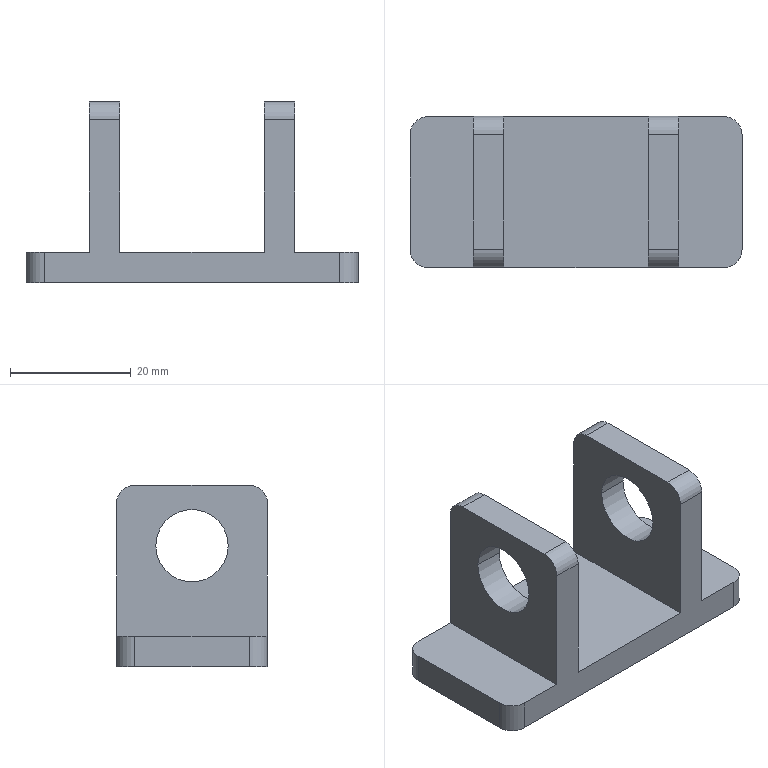Part | STEP file | Hinge top seat 3 | 1 solid | 26 faces | box 55 x 25 x 30 mm | volume 11917 mm3 | plane 14 | cylinder 12 | commonest cylinder face diameters 6 x8 12 x4
STEP:
#1=CARTESIAN_POINT('',(-12.,6.,20.));
#2=VERTEX_POINT('',#1);
#3=CARTESIAN_POINT('',(-12.,-6.,20.));
#4=VERTEX_POINT('',#3);
#5=CARTESIAN_POINT('',(-12.,0.,20.));
#6=DIRECTION('',(-1.,0.,0.));
#7=DIRECTION('',(0.,-1.,0.));
#8=AXIS2_PLACEMENT_3D('',#5,#6,#7);
#9=CIRCLE('',#8,6.);
#10=EDGE_CURVE('',#2,#4,#9,.T.);
#11=ORIENTED_EDGE('',*,*,#10,.F.);
#12=CARTESIAN_POINT('',(-17.,6.,20.));
#13=VERTEX_POINT('',#12);
#14=CARTESIAN_POINT('',(27.5,6.,20.));
#15=DIRECTION('',(-1.,0.,0.));
#16=VECTOR('',#15,1000.);
#17=LINE('',#14,#16);
#18=EDGE_CURVE('',#2,#13,#17,.T.);
#19=ORIENTED_EDGE('',*,*,#18,.T.);
#20=CARTESIAN_POINT('',(-17.,-6.,20.));
#21=VERTEX_POINT('',#20);
#22=CARTESIAN_POINT('',(-17.,0.,20.));
#23=DIRECTION('',(-1.,0.,0.));
#24=DIRECTION('',(0.,-1.,0.));
#25=AXIS2_PLACEMENT_3D('',#22,#23,#24);
#26=CIRCLE('',#25,6.);
#27=EDGE_CURVE('',#13,#21,#26,.T.);
#28=ORIENTED_EDGE('',*,*,#27,.T.);
#29=CARTESIAN_POINT('',(27.5,-6.,20.));
#30=DIRECTION('',(-1.,0.,0.));
#31=VECTOR('',#30,1000.);
#32=LINE('',#29,#31);
#33=EDGE_CURVE('',#4,#21,#32,.T.);
#34=ORIENTED_EDGE('',*,*,#33,.F.);
#35=EDGE_LOOP('',(#11,#19,#28,#34));
#36=FACE_OUTER_BOUND('',#35,.T.);
#37=CARTESIAN_POINT('',(27.5,0.,20.));
#38=DIRECTION('',(-1.,0.,0.));
#39=DIRECTION('',(0.,-1.,0.));
#40=AXIS2_PLACEMENT_3D('',#37,#38,#39);
#41=CYLINDRICAL_SURFACE('',#40,6.);
#42=ADVANCED_FACE('',(#36),#41,.F.);
#43=CARTESIAN_POINT('',(17.,6.,20.));
#44=VERTEX_POINT('',#43);
#45=CARTESIAN_POINT('',(17.,-6.,20.));
#46=VERTEX_POINT('',#45);
#47=CARTESIAN_POINT('',(17.,0.,20.));
#48=DIRECTION('',(-1.,0.,0.));
#49=DIRECTION('',(0.,-1.,0.));
#50=AXIS2_PLACEMENT_3D('',#47,#48,#49);
#51=CIRCLE('',#50,6.);
#52=EDGE_CURVE('',#44,#46,#51,.T.);
#53=ORIENTED_EDGE('',*,*,#52,.F.);
#54=CARTESIAN_POINT('',(12.,6.,20.));
#55=VERTEX_POINT('',#54);
#56=CARTESIAN_POINT('',(27.5,6.,20.));
#57=DIRECTION('',(-1.,0.,0.));
#58=VECTOR('',#57,1000.);
#59=LINE('',#56,#58);
#60=EDGE_CURVE('',#44,#55,#59,.T.);
#61=ORIENTED_EDGE('',*,*,#60,.T.);
#62=CARTESIAN_POINT('',(12.,-6.,20.));
#63=VERTEX_POINT('',#62);
#64=CARTESIAN_POINT('',(12.,0.,20.));
#65=DIRECTION('',(1.,0.,0.));
#66=DIRECTION('',(0.,0.,-1.));
#67=AXIS2_PLACEMENT_3D('',#64,#65,#66);
#68=CIRCLE('',#67,6.);
#69=EDGE_CURVE('',#63,#55,#68,.T.);
#70=ORIENTED_EDGE('',*,*,#69,.F.);
#71=CARTESIAN_POINT('',(27.5,-6.,20.));
#72=DIRECTION('',(-1.,0.,0.));
#73=VECTOR('',#72,1000.);
#74=LINE('',#71,#73);
#75=EDGE_CURVE('',#46,#63,#74,.T.);
#76=ORIENTED_EDGE('',*,*,#75,.F.);
#77=EDGE_LOOP('',(#53,#61,#70,#76));
#78=FACE_OUTER_BOUND('',#77,.T.);
#79=CARTESIAN_POINT('',(27.5,0.,20.));
#80=DIRECTION('',(-1.,0.,0.));
#81=DIRECTION('',(0.,-1.,0.));
#82=AXIS2_PLACEMENT_3D('',#79,#80,#81);
#83=CYLINDRICAL_SURFACE('',#82,6.);
#84=ADVANCED_FACE('',(#78),#83,.F.);
#85=CARTESIAN_POINT('',(17.,-12.5,5.));
#86=VERTEX_POINT('',#85);
#87=CARTESIAN_POINT('',(24.5,-12.5,5.));
#88=VERTEX_POINT('',#87);
#89=CARTESIAN_POINT('',(-27.5,-12.5,5.));
#90=DIRECTION('',(1.,0.,0.));
#91=VECTOR('',#90,1000.);
#92=LINE('',#89,#91);
#93=EDGE_CURVE('',#86,#88,#92,.T.);
#94=ORIENTED_EDGE('',*,*,#93,.T.);
#95=CARTESIAN_POINT('',(27.5,-9.5,5.));
#96=VERTEX_POINT('',#95);
#97=CARTESIAN_POINT('',(24.5,-9.5,5.));
#98=DIRECTION('',(0.,0.,1.));
#99=DIRECTION('',(1.,0.,0.));
#100=AXIS2_PLACEMENT_3D('',#97,#98,#99);
#101=CIRCLE('',#100,3.);
#102=EDGE_CURVE('',#88,#96,#101,.T.);
#103=ORIENTED_EDGE('',*,*,#102,.T.);
#104=CARTESIAN_POINT('',(27.5,9.5,5.));
#105=VERTEX_POINT('',#104);
#106=CARTESIAN_POINT('',(27.5,12.5,5.));
#107=DIRECTION('',(0.,1.,0.));
#108=VECTOR('',#107,1000.);
#109=LINE('',#106,#108);
#110=EDGE_CURVE('',#96,#105,#109,.T.);
#111=ORIENTED_EDGE('',*,*,#110,.T.);
#112=CARTESIAN_POINT('',(24.5,12.5,5.));
#113=VERTEX_POINT('',#112);
#114=CARTESIAN_POINT('',(24.5,9.5,5.));
#115=DIRECTION('',(0.,0.,1.));
#116=DIRECTION('',(1.,0.,0.));
#117=AXIS2_PLACEMENT_3D('',#114,#115,#116);
#118=CIRCLE('',#117,3.);
#119=EDGE_CURVE('',#105,#113,#118,.T.);
#120=ORIENTED_EDGE('',*,*,#119,.T.);
#121=CARTESIAN_POINT('',(17.,12.5,5.));
#122=VERTEX_POINT('',#121);
#123=CARTESIAN_POINT('',(-27.5,12.5,5.));
#124=DIRECTION('',(-1.,0.,0.));
#125=VECTOR('',#124,1000.);
#126=LINE('',#123,#125);
#127=EDGE_CURVE('',#113,#122,#126,.T.);
#128=ORIENTED_EDGE('',*,*,#127,.T.);
#129=CARTESIAN_POINT('',(17.,12.5,5.));
#130=DIRECTION('',(0.,1.,0.));
#131=VECTOR('',#130,1000.);
#132=LINE('',#129,#131);
#133=EDGE_CURVE('',#86,#122,#132,.T.);
#134=ORIENTED_EDGE('',*,*,#133,.F.);
#135=EDGE_LOOP('',(#94,#103,#111,#120,#128,#134));
#136=FACE_OUTER_BOUND('',#135,.T.);
#137=CARTESIAN_POINT('',(0.,0.,5.));
#138=DIRECTION('',(0.,0.,1.));
#139=DIRECTION('',(1.,0.,0.));
#140=AXIS2_PLACEMENT_3D('',#137,#138,#139);
#141=PLANE('',#140);
#142=ADVANCED_FACE('',(#136),#141,.T.);
#143=CARTESIAN_POINT('',(-12.,-12.5,5.));
#144=VERTEX_POINT('',#143);
#145=CARTESIAN_POINT('',(12.,-12.5,5.));
#146=VERTEX_POINT('',#145);
#147=CARTESIAN_POINT('',(-27.5,-12.5,5.));
#148=DIRECTION('',(1.,0.,0.));
#149=VECTOR('',#148,1000.);
#150=LINE('',#147,#149);
#151=EDGE_CURVE('',#144,#146,#150,.T.);
#152=ORIENTED_EDGE('',*,*,#151,.T.);
#153=CARTESIAN_POINT('',(12.,12.5,5.));
#154=VERTEX_POINT('',#153);
#155=CARTESIAN_POINT('',(12.,12.5,5.));
#156=DIRECTION('',(0.,-1.,0.));
#157=VECTOR('',#156,1000.);
#158=LINE('',#155,#157);
#159=EDGE_CURVE('',#154,#146,#158,.T.);
#160=ORIENTED_EDGE('',*,*,#159,.F.);
#161=CARTESIAN_POINT('',(-12.,12.5,5.));
#162=VERTEX_POINT('',#161);
#163=CARTESIAN_POINT('',(-27.5,12.5,5.));
#164=DIRECTION('',(-1.,0.,0.));
#165=VECTOR('',#164,1000.);
#166=LINE('',#163,#165);
#167=EDGE_CURVE('',#154,#162,#166,.T.);
#168=ORIENTED_EDGE('',*,*,#167,.T.);
#169=CARTESIAN_POINT('',(-12.,12.5,5.));
#170=DIRECTION('',(0.,1.,0.));
#171=VECTOR('',#170,1000.);
#172=LINE('',#169,#171);
#173=EDGE_CURVE('',#144,#162,#172,.T.);
#174=ORIENTED_EDGE('',*,*,#173,.F.);
#175=EDGE_LOOP('',(#152,#160,#168,#174));
#176=FACE_OUTER_BOUND('',#175,.T.);
#177=CARTESIAN_POINT('',(0.,0.,5.));
#178=DIRECTION('',(0.,0.,1.));
#179=DIRECTION('',(1.,0.,0.));
#180=AXIS2_PLACEMENT_3D('',#177,#178,#179);
#181=PLANE('',#180);
#182=ADVANCED_FACE('',(#176),#181,.T.);
#183=ORIENTED_EDGE('',*,*,#110,.F.);
#184=CARTESIAN_POINT('',(27.5,-9.5,0.));
#185=VERTEX_POINT('',#184);
#186=CARTESIAN_POINT('',(27.5,-9.5,5.));
#187=DIRECTION('',(0.,0.,-1.));
#188=VECTOR('',#187,1000.);
#189=LINE('',#186,#188);
#190=EDGE_CURVE('',#96,#185,#189,.T.);
#191=ORIENTED_EDGE('',*,*,#190,.T.);
#192=CARTESIAN_POINT('',(27.5,9.5,0.));
#193=VERTEX_POINT('',#192);
#194=CARTESIAN_POINT('',(27.5,12.5,0.));
#195=DIRECTION('',(0.,1.,0.));
#196=VECTOR('',#195,1000.);
#197=LINE('',#194,#196);
#198=EDGE_CURVE('',#185,#193,#197,.T.);
#199=ORIENTED_EDGE('',*,*,#198,.T.);
#200=CARTESIAN_POINT('',(27.5,9.5,5.));
#201=DIRECTION('',(0.,0.,1.));
#202=VECTOR('',#201,1000.);
#203=LINE('',#200,#202);
#204=EDGE_CURVE('',#193,#105,#203,.T.);
#205=ORIENTED_EDGE('',*,*,#204,.T.);
#206=EDGE_LOOP('',(#183,#191,#199,#205));
#207=FACE_OUTER_BOUND('',#206,.T.);
#208=CARTESIAN_POINT('',(27.5,12.5,5.));
#209=DIRECTION('',(-1.,0.,0.));
#210=DIRECTION('',(0.,-1.,0.));
#211=AXIS2_PLACEMENT_3D('',#208,#209,#210);
#212=PLANE('',#211);
#213=ADVANCED_FACE('',(#207),#212,.F.);
#214=ORIENTED_EDGE('',*,*,#127,.F.);
#215=CARTESIAN_POINT('',(24.5,12.5,0.));
#216=VERTEX_POINT('',#215);
#217=CARTESIAN_POINT('',(24.5,12.5,5.));
#218=DIRECTION('',(0.,0.,-1.));
#219=VECTOR('',#218,1000.);
#220=LINE('',#217,#219);
#221=EDGE_CURVE('',#113,#216,#220,.T.);
#222=ORIENTED_EDGE('',*,*,#221,.T.);
#223=CARTESIAN_POINT('',(-24.5,12.5,0.));
#224=VERTEX_POINT('',#223);
#225=CARTESIAN_POINT('',(-27.5,12.5,0.));
#226=DIRECTION('',(-1.,0.,0.));
#227=VECTOR('',#226,1000.);
#228=LINE('',#225,#227);
#229=EDGE_CURVE('',#216,#224,#228,.T.);
#230=ORIENTED_EDGE('',*,*,#229,.T.);
#231=CARTESIAN_POINT('',(-24.5,12.5,5.));
#232=VERTEX_POINT('',#231);
#233=CARTESIAN_POINT('',(-24.5,12.5,5.));
#234=DIRECTION('',(0.,0.,1.));
#235=VECTOR('',#234,1000.);
#236=LINE('',#233,#235);
#237=EDGE_CURVE('',#224,#232,#236,.T.);
#238=ORIENTED_EDGE('',*,*,#237,.T.);
#239=CARTESIAN_POINT('',(-17.,12.5,5.));
#240=VERTEX_POINT('',#239);
#241=CARTESIAN_POINT('',(-27.5,12.5,5.));
#242=DIRECTION('',(-1.,0.,0.));
#243=VECTOR('',#242,1000.);
#244=LINE('',#241,#243);
#245=EDGE_CURVE('',#240,#232,#244,.T.);
#246=ORIENTED_EDGE('',*,*,#245,.F.);
#247=CARTESIAN_POINT('',(-17.,12.5,27.));
#248=VERTEX_POINT('',#247);
#249=CARTESIAN_POINT('',(-17.,12.5,30.));
#250=DIRECTION('',(0.,0.,-1.));
#251=VECTOR('',#250,1000.);
#252=LINE('',#249,#251);
#253=EDGE_CURVE('',#248,#240,#252,.T.);
#254=ORIENTED_EDGE('',*,*,#253,.F.);
#255=CARTESIAN_POINT('',(-12.,12.5,27.));
#256=VERTEX_POINT('',#255);
#257=CARTESIAN_POINT('',(-12.,12.5,27.));
#258=DIRECTION('',(1.,0.,0.));
#259=VECTOR('',#258,1000.);
#260=LINE('',#257,#259);
#261=EDGE_CURVE('',#248,#256,#260,.T.);
#262=ORIENTED_EDGE('',*,*,#261,.T.);
#263=CARTESIAN_POINT('',(-12.,12.5,30.));
#264=DIRECTION('',(0.,0.,-1.));
#265=VECTOR('',#264,1000.);
#266=LINE('',#263,#265);
#267=EDGE_CURVE('',#256,#162,#266,.T.);
#268=ORIENTED_EDGE('',*,*,#267,.T.);
#269=ORIENTED_EDGE('',*,*,#167,.F.);
#270=CARTESIAN_POINT('',(12.,12.5,27.));
#271=VERTEX_POINT('',#270);
#272=CARTESIAN_POINT('',(12.,12.5,30.));
#273=DIRECTION('',(0.,0.,-1.));
#274=VECTOR('',#273,1000.);
#275=LINE('',#272,#274);
#276=EDGE_CURVE('',#271,#154,#275,.T.);
#277=ORIENTED_EDGE('',*,*,#276,.F.);
#278=CARTESIAN_POINT('',(17.,12.5,27.));
#279=VERTEX_POINT('',#278);
#280=CARTESIAN_POINT('',(-27.5,12.5,27.));
#281=DIRECTION('',(1.,0.,0.));
#282=VECTOR('',#281,1000.);
#283=LINE('',#280,#282);
#284=EDGE_CURVE('',#271,#279,#283,.T.);
#285=ORIENTED_EDGE('',*,*,#284,.T.);
#286=CARTESIAN_POINT('',(17.,12.5,30.));
#287=DIRECTION('',(0.,0.,-1.));
#288=VECTOR('',#287,1000.);
#289=LINE('',#286,#288);
#290=EDGE_CURVE('',#279,#122,#289,.T.);
#291=ORIENTED_EDGE('',*,*,#290,.T.);
#292=EDGE_LOOP('',(#214,#222,#230,#238,#246,#254,#262,#268,#269,#277,#285,#291));
#293=FACE_OUTER_BOUND('',#292,.T.);
#294=CARTESIAN_POINT('',(-27.5,12.5,5.));
#295=DIRECTION('',(0.,-1.,0.));
#296=DIRECTION('',(0.,0.,-1.));
#297=AXIS2_PLACEMENT_3D('',#294,#295,#296);
#298=PLANE('',#297);
#299=ADVANCED_FACE('',(#293),#298,.F.);
#300=CARTESIAN_POINT('',(-27.5,9.5,5.));
#301=VERTEX_POINT('',#300);
#302=CARTESIAN_POINT('',(-27.5,-9.5,5.));
#303=VERTEX_POINT('',#302);
#304=CARTESIAN_POINT('',(-27.5,12.5,5.));
#305=DIRECTION('',(0.,-1.,0.));
#306=VECTOR('',#305,1000.);
#307=LINE('',#304,#306);
#308=EDGE_CURVE('',#301,#303,#307,.T.);
#309=ORIENTED_EDGE('',*,*,#308,.F.);
#310=CARTESIAN_POINT('',(-27.5,9.5,0.));
#311=VERTEX_POINT('',#310);
#312=CARTESIAN_POINT('',(-27.5,9.5,5.));
#313=DIRECTION('',(0.,0.,-1.));
#314=VECTOR('',#313,1000.);
#315=LINE('',#312,#314);
#316=EDGE_CURVE('',#301,#311,#315,.T.);
#317=ORIENTED_EDGE('',*,*,#316,.T.);
#318=CARTESIAN_POINT('',(-27.5,-9.5,0.));
#319=VERTEX_POINT('',#318);
#320=CARTESIAN_POINT('',(-27.5,12.5,0.));
#321=DIRECTION('',(0.,-1.,0.));
#322=VECTOR('',#321,1000.);
#323=LINE('',#320,#322);
#324=EDGE_CURVE('',#311,#319,#323,.T.);
#325=ORIENTED_EDGE('',*,*,#324,.T.);
#326=CARTESIAN_POINT('',(-27.5,-9.5,5.));
#327=DIRECTION('',(0.,0.,1.));
#328=VECTOR('',#327,1000.);
#329=LINE('',#326,#328);
#330=EDGE_CURVE('',#319,#303,#329,.T.);
#331=ORIENTED_EDGE('',*,*,#330,.T.);
#332=EDGE_LOOP('',(#309,#317,#325,#331));
#333=FACE_OUTER_BOUND('',#332,.T.);
#334=CARTESIAN_POINT('',(-27.5,12.5,5.));
#335=DIRECTION('',(1.,0.,0.));
#336=DIRECTION('',(0.,0.,-1.));
#337=AXIS2_PLACEMENT_3D('',#334,#335,#336);
#338=PLANE('',#337);
#339=ADVANCED_FACE('',(#333),#338,.F.);
#340=CARTESIAN_POINT('',(-24.5,-12.5,0.));
#341=VERTEX_POINT('',#340);
#342=CARTESIAN_POINT('',(24.5,-12.5,0.));
#343=VERTEX_POINT('',#342);
#344=CARTESIAN_POINT('',(-27.5,-12.5,0.));
#345=DIRECTION('',(1.,0.,0.));
#346=VECTOR('',#345,1000.);
#347=LINE('',#344,#346);
#348=EDGE_CURVE('',#341,#343,#347,.T.);
#349=ORIENTED_EDGE('',*,*,#348,.T.);
#350=CARTESIAN_POINT('',(24.5,-12.5,5.));
#351=DIRECTION('',(0.,0.,1.));
#352=VECTOR('',#351,1000.);
#353=LINE('',#350,#352);
#354=EDGE_CURVE('',#343,#88,#353,.T.);
#355=ORIENTED_EDGE('',*,*,#354,.T.);
#356=ORIENTED_EDGE('',*,*,#93,.F.);
#357=CARTESIAN_POINT('',(17.,-12.5,27.));
#358=VERTEX_POINT('',#357);
#359=CARTESIAN_POINT('',(17.,-12.5,30.));
#360=DIRECTION('',(0.,0.,-1.));
#361=VECTOR('',#360,1000.);
#362=LINE('',#359,#361);
#363=EDGE_CURVE('',#358,#86,#362,.T.);
#364=ORIENTED_EDGE('',*,*,#363,.F.);
#365=CARTESIAN_POINT('',(12.,-12.5,27.));
#366=VERTEX_POINT('',#365);
#367=CARTESIAN_POINT('',(-27.5,-12.5,27.));
#368=DIRECTION('',(-1.,0.,0.));
#369=VECTOR('',#368,1000.);
#370=LINE('',#367,#369);
#371=EDGE_CURVE('',#358,#366,#370,.T.);
#372=ORIENTED_EDGE('',*,*,#371,.T.);
#373=CARTESIAN_POINT('',(12.,-12.5,30.));
#374=DIRECTION('',(0.,0.,-1.));
#375=VECTOR('',#374,1000.);
#376=LINE('',#373,#375);
#377=EDGE_CURVE('',#366,#146,#376,.T.);
#378=ORIENTED_EDGE('',*,*,#377,.T.);
#379=ORIENTED_EDGE('',*,*,#151,.F.);
#380=CARTESIAN_POINT('',(-12.,-12.5,27.));
#381=VERTEX_POINT('',#380);
#382=CARTESIAN_POINT('',(-12.,-12.5,30.));
#383=DIRECTION('',(0.,0.,-1.));
#384=VECTOR('',#383,1000.);
#385=LINE('',#382,#384);
#386=EDGE_CURVE('',#381,#144,#385,.T.);
#387=ORIENTED_EDGE('',*,*,#386,.F.);
#388=CARTESIAN_POINT('',(-17.,-12.5,27.));
#389=VERTEX_POINT('',#388);
#390=CARTESIAN_POINT('',(-17.,-12.5,27.));
#391=DIRECTION('',(-1.,0.,0.));
#392=VECTOR('',#391,1000.);
#393=LINE('',#390,#392);
#394=EDGE_CURVE('',#381,#389,#393,.T.);
#395=ORIENTED_EDGE('',*,*,#394,.T.);
#396=CARTESIAN_POINT('',(-17.,-12.5,5.));
#397=VERTEX_POINT('',#396);
#398=CARTESIAN_POINT('',(-17.,-12.5,30.));
#399=DIRECTION('',(0.,0.,-1.));
#400=VECTOR('',#399,1000.);
#401=LINE('',#398,#400);
#402=EDGE_CURVE('',#389,#397,#401,.T.);
#403=ORIENTED_EDGE('',*,*,#402,.T.);
#404=CARTESIAN_POINT('',(-24.5,-12.5,5.));
#405=VERTEX_POINT('',#404);
#406=CARTESIAN_POINT('',(-27.5,-12.5,5.));
#407=DIRECTION('',(1.,0.,0.));
#408=VECTOR('',#407,1000.);
#409=LINE('',#406,#408);
#410=EDGE_CURVE('',#405,#397,#409,.T.);
#411=ORIENTED_EDGE('',*,*,#410,.F.);
#412=CARTESIAN_POINT('',(-24.5,-12.5,5.));
#413=DIRECTION('',(0.,0.,-1.));
#414=VECTOR('',#413,1000.);
#415=LINE('',#412,#414);
#416=EDGE_CURVE('',#405,#341,#415,.T.);
#417=ORIENTED_EDGE('',*,*,#416,.T.);
#418=EDGE_LOOP('',(#349,#355,#356,#364,#372,#378,#379,#387,#395,#403,#411,#417));
#419=FACE_OUTER_BOUND('',#418,.T.);
#420=CARTESIAN_POINT('',(-27.5,-12.5,5.));
#421=DIRECTION('',(0.,1.,0.));
#422=DIRECTION('',(0.,0.,1.));
#423=AXIS2_PLACEMENT_3D('',#420,#421,#422);
#424=PLANE('',#423);
#425=ADVANCED_FACE('',(#419),#424,.F.);
#426=ORIENTED_EDGE('',*,*,#245,.T.);
#427=CARTESIAN_POINT('',(-24.5,9.5,5.));
#428=DIRECTION('',(0.,0.,1.));
#429=DIRECTION('',(1.,0.,0.));
#430=AXIS2_PLACEMENT_3D('',#427,#428,#429);
#431=CIRCLE('',#430,3.);
#432=EDGE_CURVE('',#232,#301,#431,.T.);
#433=ORIENTED_EDGE('',*,*,#432,.T.);
#434=ORIENTED_EDGE('',*,*,#308,.T.);
#435=CARTESIAN_POINT('',(-24.5,-9.5,5.));
#436=DIRECTION('',(0.,0.,1.));
#437=DIRECTION('',(1.,0.,0.));
#438=AXIS2_PLACEMENT_3D('',#435,#436,#437);
#439=CIRCLE('',#438,3.);
#440=EDGE_CURVE('',#303,#405,#439,.T.);
#441=ORIENTED_EDGE('',*,*,#440,.T.);
#442=ORIENTED_EDGE('',*,*,#410,.T.);
#443=CARTESIAN_POINT('',(-17.,12.5,5.));
#444=DIRECTION('',(0.,-1.,0.));
#445=VECTOR('',#444,1000.);
#446=LINE('',#443,#445);
#447=EDGE_CURVE('',#240,#397,#446,.T.);
#448=ORIENTED_EDGE('',*,*,#447,.F.);
#449=EDGE_LOOP('',(#426,#433,#434,#441,#442,#448));
#450=FACE_OUTER_BOUND('',#449,.T.);
#451=CARTESIAN_POINT('',(0.,0.,5.));
#452=DIRECTION('',(0.,0.,1.));
#453=DIRECTION('',(1.,0.,0.));
#454=AXIS2_PLACEMENT_3D('',#451,#452,#453);
#455=PLANE('',#454);
#456=ADVANCED_FACE('',(#450),#455,.T.);
#457=ORIENTED_EDGE('',*,*,#198,.F.);
#458=CARTESIAN_POINT('',(24.5,-9.5,0.));
#459=DIRECTION('',(0.,0.,-1.));
#460=DIRECTION('',(1.,0.,0.));
#461=AXIS2_PLACEMENT_3D('',#458,#459,#460);
#462=CIRCLE('',#461,3.);
#463=EDGE_CURVE('',#185,#343,#462,.T.);
#464=ORIENTED_EDGE('',*,*,#463,.T.);
#465=ORIENTED_EDGE('',*,*,#348,.F.);
#466=CARTESIAN_POINT('',(-24.5,-9.5,0.));
#467=DIRECTION('',(0.,0.,-1.));
#468=DIRECTION('',(1.,0.,0.));
#469=AXIS2_PLACEMENT_3D('',#466,#467,#468);
#470=CIRCLE('',#469,3.);
#471=EDGE_CURVE('',#341,#319,#470,.T.);
#472=ORIENTED_EDGE('',*,*,#471,.T.);
#473=ORIENTED_EDGE('',*,*,#324,.F.);
#474=CARTESIAN_POINT('',(-24.5,9.5,0.));
#475=DIRECTION('',(0.,0.,-1.));
#476=DIRECTION('',(1.,0.,0.));
#477=AXIS2_PLACEMENT_3D('',#474,#475,#476);
#478=CIRCLE('',#477,3.);
#479=EDGE_CURVE('',#311,#224,#478,.T.);
#480=ORIENTED_EDGE('',*,*,#479,.T.);
#481=ORIENTED_EDGE('',*,*,#229,.F.);
#482=CARTESIAN_POINT('',(24.5,9.5,0.));
#483=DIRECTION('',(0.,0.,-1.));
#484=DIRECTION('',(1.,0.,0.));
#485=AXIS2_PLACEMENT_3D('',#482,#483,#484);
#486=CIRCLE('',#485,3.);
#487=EDGE_CURVE('',#216,#193,#486,.T.);
#488=ORIENTED_EDGE('',*,*,#487,.T.);
#489=EDGE_LOOP('',(#457,#464,#465,#472,#473,#480,#481,#488));
#490=FACE_OUTER_BOUND('',#489,.T.);
#491=CARTESIAN_POINT('',(0.,0.,0.));
#492=DIRECTION('',(0.,0.,1.));
#493=DIRECTION('',(1.,0.,0.));
#494=AXIS2_PLACEMENT_3D('',#491,#492,#493);
#495=PLANE('',#494);
#496=ADVANCED_FACE('',(#490),#495,.F.);
#497=CARTESIAN_POINT('',(-12.,0.,20.));
#498=DIRECTION('',(-1.,0.,0.));
#499=DIRECTION('',(0.,-1.,0.));
#500=AXIS2_PLACEMENT_3D('',#497,#498,#499);
#501=CIRCLE('',#500,6.);
#502=EDGE_CURVE('',#4,#2,#501,.T.);
#503=ORIENTED_EDGE('',*,*,#502,.T.);
#504=ORIENTED_EDGE('',*,*,#10,.T.);
#505=EDGE_LOOP('',(#503,#504));
#506=FACE_BOUND('',#505,.T.);
#507=CARTESIAN_POINT('',(-12.,-9.5,30.));
#508=VERTEX_POINT('',#507);
#509=CARTESIAN_POINT('',(-12.,9.5,30.));
#510=VERTEX_POINT('',#509);
#511=CARTESIAN_POINT('',(-12.,12.5,30.));
#512=DIRECTION('',(0.,1.,0.));
#513=VECTOR('',#512,1000.);
#514=LINE('',#511,#513);
#515=EDGE_CURVE('',#508,#510,#514,.T.);
#516=ORIENTED_EDGE('',*,*,#515,.F.);
#517=CARTESIAN_POINT('',(-12.,-9.5,27.));
#518=DIRECTION('',(1.,0.,0.));
#519=DIRECTION('',(0.,-1.,0.));
#520=AXIS2_PLACEMENT_3D('',#517,#518,#519);
#521=CIRCLE('',#520,3.);
#522=EDGE_CURVE('',#508,#381,#521,.T.);
#523=ORIENTED_EDGE('',*,*,#522,.T.);
#524=ORIENTED_EDGE('',*,*,#386,.T.);
#525=ORIENTED_EDGE('',*,*,#173,.T.);
#526=ORIENTED_EDGE('',*,*,#267,.F.);
#527=CARTESIAN_POINT('',(-12.,9.5,27.));
#528=DIRECTION('',(1.,0.,0.));
#529=DIRECTION('',(0.,-1.,0.));
#530=AXIS2_PLACEMENT_3D('',#527,#528,#529);
#531=CIRCLE('',#530,3.);
#532=EDGE_CURVE('',#256,#510,#531,.T.);
#533=ORIENTED_EDGE('',*,*,#532,.T.);
#534=EDGE_LOOP('',(#516,#523,#524,#525,#526,#533));
#535=FACE_OUTER_BOUND('',#534,.T.);
#536=CARTESIAN_POINT('',(-12.,12.5,30.));
#537=DIRECTION('',(-1.,0.,0.));
#538=DIRECTION('',(0.,-1.,0.));
#539=AXIS2_PLACEMENT_3D('',#536,#537,#538);
#540=PLANE('',#539);
#541=ADVANCED_FACE('',(#506,#535),#540,.F.);
#542=CARTESIAN_POINT('',(-17.,0.,20.));
#543=DIRECTION('',(-1.,0.,0.));
#544=DIRECTION('',(0.,-1.,0.));
#545=AXIS2_PLACEMENT_3D('',#542,#543,#544);
#546=CIRCLE('',#545,6.);
#547=EDGE_CURVE('',#21,#13,#546,.T.);
#548=ORIENTED_EDGE('',*,*,#547,.F.);
#549=ORIENTED_EDGE('',*,*,#27,.F.);
#550=EDGE_LOOP('',(#548,#549));
#551=FACE_BOUND('',#550,.T.);
#552=ORIENTED_EDGE('',*,*,#402,.F.);
#553=CARTESIAN_POINT('',(-17.,-9.5,30.));
#554=VERTEX_POINT('',#553);
#555=CARTESIAN_POINT('',(-17.,-9.5,27.));
#556=DIRECTION('',(-1.,0.,0.));
#557=DIRECTION('',(0.,1.,0.));
#558=AXIS2_PLACEMENT_3D('',#555,#556,#557);
#559=CIRCLE('',#558,3.);
#560=EDGE_CURVE('',#389,#554,#559,.T.);
#561=ORIENTED_EDGE('',*,*,#560,.T.);
#562=CARTESIAN_POINT('',(-17.,9.5,30.));
#563=VERTEX_POINT('',#562);
#564=CARTESIAN_POINT('',(-17.,12.5,30.));
#565=DIRECTION('',(0.,-1.,0.));
#566=VECTOR('',#565,1000.);
#567=LINE('',#564,#566);
#568=EDGE_CURVE('',#563,#554,#567,.T.);
#569=ORIENTED_EDGE('',*,*,#568,.F.);
#570=CARTESIAN_POINT('',(-17.,9.5,27.));
#571=DIRECTION('',(-1.,0.,0.));
#572=DIRECTION('',(0.,1.,0.));
#573=AXIS2_PLACEMENT_3D('',#570,#571,#572);
#574=CIRCLE('',#573,3.);
#575=EDGE_CURVE('',#563,#248,#574,.T.);
#576=ORIENTED_EDGE('',*,*,#575,.T.);
#577=ORIENTED_EDGE('',*,*,#253,.T.);
#578=ORIENTED_EDGE('',*,*,#447,.T.);
#579=EDGE_LOOP('',(#552,#561,#569,#576,#577,#578));
#580=FACE_OUTER_BOUND('',#579,.T.);
#581=CARTESIAN_POINT('',(-17.,12.5,30.));
#582=DIRECTION('',(1.,0.,0.));
#583=DIRECTION('',(0.,1.,0.));
#584=AXIS2_PLACEMENT_3D('',#581,#582,#583);
#585=PLANE('',#584);
#586=ADVANCED_FACE('',(#551,#580),#585,.F.);
#587=ORIENTED_EDGE('',*,*,#568,.T.);
#588=CARTESIAN_POINT('',(-12.,-9.5,30.));
#589=DIRECTION('',(1.,0.,0.));
#590=VECTOR('',#589,1000.);
#591=LINE('',#588,#590);
#592=EDGE_CURVE('',#554,#508,#591,.T.);
#593=ORIENTED_EDGE('',*,*,#592,.T.);
#594=ORIENTED_EDGE('',*,*,#515,.T.);
#595=CARTESIAN_POINT('',(-17.,9.5,30.));
#596=DIRECTION('',(-1.,0.,0.));
#597=VECTOR('',#596,1000.);
#598=LINE('',#595,#597);
#599=EDGE_CURVE('',#510,#563,#598,.T.);
#600=ORIENTED_EDGE('',*,*,#599,.T.);
#601=EDGE_LOOP('',(#587,#593,#594,#600));
#602=FACE_OUTER_BOUND('',#601,.T.);
#603=CARTESIAN_POINT('',(0.,0.,30.));
#604=DIRECTION('',(0.,0.,1.));
#605=DIRECTION('',(1.,0.,0.));
#606=AXIS2_PLACEMENT_3D('',#603,#604,#605);
#607=PLANE('',#606);
#608=ADVANCED_FACE('',(#602),#607,.T.);
#609=CARTESIAN_POINT('',(17.,0.,20.));
#610=DIRECTION('',(-1.,0.,0.));
#611=DIRECTION('',(0.,-1.,0.));
#612=AXIS2_PLACEMENT_3D('',#609,#610,#611);
#613=CIRCLE('',#612,6.);
#614=EDGE_CURVE('',#46,#44,#613,.T.);
#615=ORIENTED_EDGE('',*,*,#614,.T.);
#616=ORIENTED_EDGE('',*,*,#52,.T.);
#617=EDGE_LOOP('',(#615,#616));
#618=FACE_BOUND('',#617,.T.);
#619=ORIENTED_EDGE('',*,*,#290,.F.);
#620=CARTESIAN_POINT('',(17.,9.5,30.));
#621=VERTEX_POINT('',#620);
#622=CARTESIAN_POINT('',(17.,9.5,27.));
#623=DIRECTION('',(1.,0.,0.));
#624=DIRECTION('',(0.,-1.,0.));
#625=AXIS2_PLACEMENT_3D('',#622,#623,#624);
#626=CIRCLE('',#625,3.);
#627=EDGE_CURVE('',#279,#621,#626,.T.);
#628=ORIENTED_EDGE('',*,*,#627,.T.);
#629=CARTESIAN_POINT('',(17.,-9.5,30.));
#630=VERTEX_POINT('',#629);
#631=CARTESIAN_POINT('',(17.,12.5,30.));
#632=DIRECTION('',(0.,1.,0.));
#633=VECTOR('',#632,1000.);
#634=LINE('',#631,#633);
#635=EDGE_CURVE('',#630,#621,#634,.T.);
#636=ORIENTED_EDGE('',*,*,#635,.F.);
#637=CARTESIAN_POINT('',(17.,-9.5,27.));
#638=DIRECTION('',(1.,0.,0.));
#639=DIRECTION('',(0.,-1.,0.));
#640=AXIS2_PLACEMENT_3D('',#637,#638,#639);
#641=CIRCLE('',#640,3.);
#642=EDGE_CURVE('',#630,#358,#641,.T.);
#643=ORIENTED_EDGE('',*,*,#642,.T.);
#644=ORIENTED_EDGE('',*,*,#363,.T.);
#645=ORIENTED_EDGE('',*,*,#133,.T.);
#646=EDGE_LOOP('',(#619,#628,#636,#643,#644,#645));
#647=FACE_OUTER_BOUND('',#646,.T.);
#648=CARTESIAN_POINT('',(17.,12.5,30.));
#649=DIRECTION('',(-1.,0.,0.));
#650=DIRECTION('',(0.,-1.,0.));
#651=AXIS2_PLACEMENT_3D('',#648,#649,#650);
#652=PLANE('',#651);
#653=ADVANCED_FACE('',(#618,#647),#652,.F.);
#654=ORIENTED_EDGE('',*,*,#69,.T.);
#655=CARTESIAN_POINT('',(12.,0.,20.));
#656=DIRECTION('',(1.,0.,0.));
#657=DIRECTION('',(0.,0.,-1.));
#658=AXIS2_PLACEMENT_3D('',#655,#656,#657);
#659=CIRCLE('',#658,6.);
#660=EDGE_CURVE('',#55,#63,#659,.T.);
#661=ORIENTED_EDGE('',*,*,#660,.T.);
#662=EDGE_LOOP('',(#654,#661));
#663=FACE_BOUND('',#662,.T.);
#664=CARTESIAN_POINT('',(12.,9.5,30.));
#665=VERTEX_POINT('',#664);
#666=CARTESIAN_POINT('',(12.,-9.5,30.));
#667=VERTEX_POINT('',#666);
#668=CARTESIAN_POINT('',(12.,12.5,30.));
#669=DIRECTION('',(0.,-1.,0.));
#670=VECTOR('',#669,1000.);
#671=LINE('',#668,#670);
#672=EDGE_CURVE('',#665,#667,#671,.T.);
#673=ORIENTED_EDGE('',*,*,#672,.F.);
#674=CARTESIAN_POINT('',(12.,9.5,27.));
#675=DIRECTION('',(-1.,0.,0.));
#676=DIRECTION('',(0.,0.,-1.));
#677=AXIS2_PLACEMENT_3D('',#674,#675,#676);
#678=CIRCLE('',#677,3.);
#679=EDGE_CURVE('',#665,#271,#678,.T.);
#680=ORIENTED_EDGE('',*,*,#679,.T.);
#681=ORIENTED_EDGE('',*,*,#276,.T.);
#682=ORIENTED_EDGE('',*,*,#159,.T.);
#683=ORIENTED_EDGE('',*,*,#377,.F.);
#684=CARTESIAN_POINT('',(12.,-9.5,27.));
#685=DIRECTION('',(-1.,0.,0.));
#686=DIRECTION('',(0.,0.,-1.));
#687=AXIS2_PLACEMENT_3D('',#684,#685,#686);
#688=CIRCLE('',#687,3.);
#689=EDGE_CURVE('',#366,#667,#688,.T.);
#690=ORIENTED_EDGE('',*,*,#689,.T.);
#691=EDGE_LOOP('',(#673,#680,#681,#682,#683,#690));
#692=FACE_OUTER_BOUND('',#691,.T.);
#693=CARTESIAN_POINT('',(12.,12.5,30.));
#694=DIRECTION('',(1.,0.,0.));
#695=DIRECTION('',(0.,0.,-1.));
#696=AXIS2_PLACEMENT_3D('',#693,#694,#695);
#697=PLANE('',#696);
#698=ADVANCED_FACE('',(#663,#692),#697,.F.);
#699=ORIENTED_EDGE('',*,*,#635,.T.);
#700=CARTESIAN_POINT('',(0.,9.5,30.));
#701=DIRECTION('',(-1.,0.,0.));
#702=VECTOR('',#701,1000.);
#703=LINE('',#700,#702);
#704=EDGE_CURVE('',#621,#665,#703,.T.);
#705=ORIENTED_EDGE('',*,*,#704,.T.);
#706=ORIENTED_EDGE('',*,*,#672,.T.);
#707=CARTESIAN_POINT('',(0.,-9.5,30.));
#708=DIRECTION('',(1.,0.,0.));
#709=VECTOR('',#708,1000.);
#710=LINE('',#707,#709);
#711=EDGE_CURVE('',#667,#630,#710,.T.);
#712=ORIENTED_EDGE('',*,*,#711,.T.);
#713=EDGE_LOOP('',(#699,#705,#706,#712));
#714=FACE_OUTER_BOUND('',#713,.T.);
#715=CARTESIAN_POINT('',(0.,0.,30.));
#716=DIRECTION('',(0.,0.,-1.));
#717=DIRECTION('',(-1.,0.,0.));
#718=AXIS2_PLACEMENT_3D('',#715,#716,#717);
#719=PLANE('',#718);
#720=ADVANCED_FACE('',(#714),#719,.F.);
#721=ORIENTED_EDGE('',*,*,#627,.F.);
#722=ORIENTED_EDGE('',*,*,#284,.F.);
#723=ORIENTED_EDGE('',*,*,#679,.F.);
#724=ORIENTED_EDGE('',*,*,#704,.F.);
#725=EDGE_LOOP('',(#721,#722,#723,#724));
#726=FACE_OUTER_BOUND('',#725,.T.);
#727=CARTESIAN_POINT('',(0.,9.5,27.));
#728=DIRECTION('',(-1.,0.,0.));
#729=DIRECTION('',(0.,0.,1.));
#730=AXIS2_PLACEMENT_3D('',#727,#728,#729);
#731=CYLINDRICAL_SURFACE('',#730,3.);
#732=ADVANCED_FACE('',(#726),#731,.T.);
#733=ORIENTED_EDGE('',*,*,#689,.F.);
#734=ORIENTED_EDGE('',*,*,#371,.F.);
#735=ORIENTED_EDGE('',*,*,#642,.F.);
#736=ORIENTED_EDGE('',*,*,#711,.F.);
#737=EDGE_LOOP('',(#733,#734,#735,#736));
#738=FACE_OUTER_BOUND('',#737,.T.);
#739=CARTESIAN_POINT('',(0.,-9.5,27.));
#740=DIRECTION('',(1.,0.,0.));
#741=DIRECTION('',(0.,0.,-1.));
#742=AXIS2_PLACEMENT_3D('',#739,#740,#741);
#743=CYLINDRICAL_SURFACE('',#742,3.);
#744=ADVANCED_FACE('',(#738),#743,.T.);
#745=ORIENTED_EDGE('',*,*,#560,.F.);
#746=ORIENTED_EDGE('',*,*,#394,.F.);
#747=ORIENTED_EDGE('',*,*,#522,.F.);
#748=ORIENTED_EDGE('',*,*,#592,.F.);
#749=EDGE_LOOP('',(#745,#746,#747,#748));
#750=FACE_OUTER_BOUND('',#749,.T.);
#751=CARTESIAN_POINT('',(0.,-9.5,27.));
#752=DIRECTION('',(-1.,0.,0.));
#753=DIRECTION('',(0.,0.,1.));
#754=AXIS2_PLACEMENT_3D('',#751,#752,#753);
#755=CYLINDRICAL_SURFACE('',#754,3.);
#756=ADVANCED_FACE('',(#750),#755,.T.);
#757=ORIENTED_EDGE('',*,*,#532,.F.);
#758=ORIENTED_EDGE('',*,*,#261,.F.);
#759=ORIENTED_EDGE('',*,*,#575,.F.);
#760=ORIENTED_EDGE('',*,*,#599,.F.);
#761=EDGE_LOOP('',(#757,#758,#759,#760));
#762=FACE_OUTER_BOUND('',#761,.T.);
#763=CARTESIAN_POINT('',(0.,9.5,27.));
#764=DIRECTION('',(1.,0.,0.));
#765=DIRECTION('',(0.,0.,-1.));
#766=AXIS2_PLACEMENT_3D('',#763,#764,#765);
#767=CYLINDRICAL_SURFACE('',#766,3.);
#768=ADVANCED_FACE('',(#762),#767,.T.);
#769=ORIENTED_EDGE('',*,*,#60,.F.);
#770=ORIENTED_EDGE('',*,*,#614,.F.);
#771=ORIENTED_EDGE('',*,*,#75,.T.);
#772=ORIENTED_EDGE('',*,*,#660,.F.);
#773=EDGE_LOOP('',(#769,#770,#771,#772));
#774=FACE_OUTER_BOUND('',#773,.T.);
#775=CARTESIAN_POINT('',(27.5,0.,20.));
#776=DIRECTION('',(-1.,0.,0.));
#777=DIRECTION('',(0.,-1.,0.));
#778=AXIS2_PLACEMENT_3D('',#775,#776,#777);
#779=CYLINDRICAL_SURFACE('',#778,6.);
#780=ADVANCED_FACE('',(#774),#779,.F.);
#781=ORIENTED_EDGE('',*,*,#18,.F.);
#782=ORIENTED_EDGE('',*,*,#502,.F.);
#783=ORIENTED_EDGE('',*,*,#33,.T.);
#784=ORIENTED_EDGE('',*,*,#547,.T.);
#785=EDGE_LOOP('',(#781,#782,#783,#784));
#786=FACE_OUTER_BOUND('',#785,.T.);
#787=CARTESIAN_POINT('',(27.5,0.,20.));
#788=DIRECTION('',(-1.,0.,0.));
#789=DIRECTION('',(0.,-1.,0.));
#790=AXIS2_PLACEMENT_3D('',#787,#788,#789);
#791=CYLINDRICAL_SURFACE('',#790,6.);
#792=ADVANCED_FACE('',(#786),#791,.F.);
#793=ORIENTED_EDGE('',*,*,#102,.F.);
#794=ORIENTED_EDGE('',*,*,#354,.F.);
#795=ORIENTED_EDGE('',*,*,#463,.F.);
#796=ORIENTED_EDGE('',*,*,#190,.F.);
#797=EDGE_LOOP('',(#793,#794,#795,#796));
#798=FACE_OUTER_BOUND('',#797,.T.);
#799=CARTESIAN_POINT('',(24.5,-9.5,5.));
#800=DIRECTION('',(0.,0.,-1.));
#801=DIRECTION('',(-1.,0.,0.));
#802=AXIS2_PLACEMENT_3D('',#799,#800,#801);
#803=CYLINDRICAL_SURFACE('',#802,3.);
#804=ADVANCED_FACE('',(#798),#803,.T.);
#805=ORIENTED_EDGE('',*,*,#119,.F.);
#806=ORIENTED_EDGE('',*,*,#204,.F.);
#807=ORIENTED_EDGE('',*,*,#487,.F.);
#808=ORIENTED_EDGE('',*,*,#221,.F.);
#809=EDGE_LOOP('',(#805,#806,#807,#808));
#810=FACE_OUTER_BOUND('',#809,.T.);
#811=CARTESIAN_POINT('',(24.5,9.5,5.));
#812=DIRECTION('',(0.,0.,-1.));
#813=DIRECTION('',(-1.,0.,0.));
#814=AXIS2_PLACEMENT_3D('',#811,#812,#813);
#815=CYLINDRICAL_SURFACE('',#814,3.);
#816=ADVANCED_FACE('',(#810),#815,.T.);
#817=ORIENTED_EDGE('',*,*,#432,.F.);
#818=ORIENTED_EDGE('',*,*,#237,.F.);
#819=ORIENTED_EDGE('',*,*,#479,.F.);
#820=ORIENTED_EDGE('',*,*,#316,.F.);
#821=EDGE_LOOP('',(#817,#818,#819,#820));
#822=FACE_OUTER_BOUND('',#821,.T.);
#823=CARTESIAN_POINT('',(-24.5,9.5,5.));
#824=DIRECTION('',(0.,0.,-1.));
#825=DIRECTION('',(-1.,0.,0.));
#826=AXIS2_PLACEMENT_3D('',#823,#824,#825);
#827=CYLINDRICAL_SURFACE('',#826,3.);
#828=ADVANCED_FACE('',(#822),#827,.T.);
#829=ORIENTED_EDGE('',*,*,#440,.F.);
#830=ORIENTED_EDGE('',*,*,#330,.F.);
#831=ORIENTED_EDGE('',*,*,#471,.F.);
#832=ORIENTED_EDGE('',*,*,#416,.F.);
#833=EDGE_LOOP('',(#829,#830,#831,#832));
#834=FACE_OUTER_BOUND('',#833,.T.);
#835=CARTESIAN_POINT('',(-24.5,-9.5,5.));
#836=DIRECTION('',(0.,0.,-1.));
#837=DIRECTION('',(-1.,0.,0.));
#838=AXIS2_PLACEMENT_3D('',#835,#836,#837);
#839=CYLINDRICAL_SURFACE('',#838,3.);
#840=ADVANCED_FACE('',(#834),#839,.T.);
#841=CLOSED_SHELL('',(#42,#84,#142,#182,#213,#299,#339,#425,#456,#496,#541,#586,#608,#653,#698,#720,#732,#744,#756,#768,#780,#792,#804,#816,#828,#840));
#842=MANIFOLD_SOLID_BREP('',#841);
#843=CARTESIAN_POINT('',(0.,0.,0.));
#844=DIRECTION('',(0.,0.,1.));
#845=DIRECTION('',(1.,0.,0.));
#846=AXIS2_PLACEMENT_3D('',#843,#844,#845);
#847=(LENGTH_UNIT()NAMED_UNIT(*)SI_UNIT(.MILLI.,.METRE.));
#848=UNCERTAINTY_MEASURE_WITH_UNIT(LENGTH_MEASURE(0.00001),#847,'','');
#849=(NAMED_UNIT(*)PLANE_ANGLE_UNIT()SI_UNIT($,.RADIAN.));
#850=(NAMED_UNIT(*)SI_UNIT($,.STERADIAN.)SOLID_ANGLE_UNIT());
#851=(GEOMETRIC_REPRESENTATION_CONTEXT(3)GLOBAL_UNCERTAINTY_ASSIGNED_CONTEXT((#848))GLOBAL_UNIT_ASSIGNED_CONTEXT((#847,#849,#850))REPRESENTATION_CONTEXT('',''));
#852=ADVANCED_BREP_SHAPE_REPRESENTATION('',(#842,#846),#851);